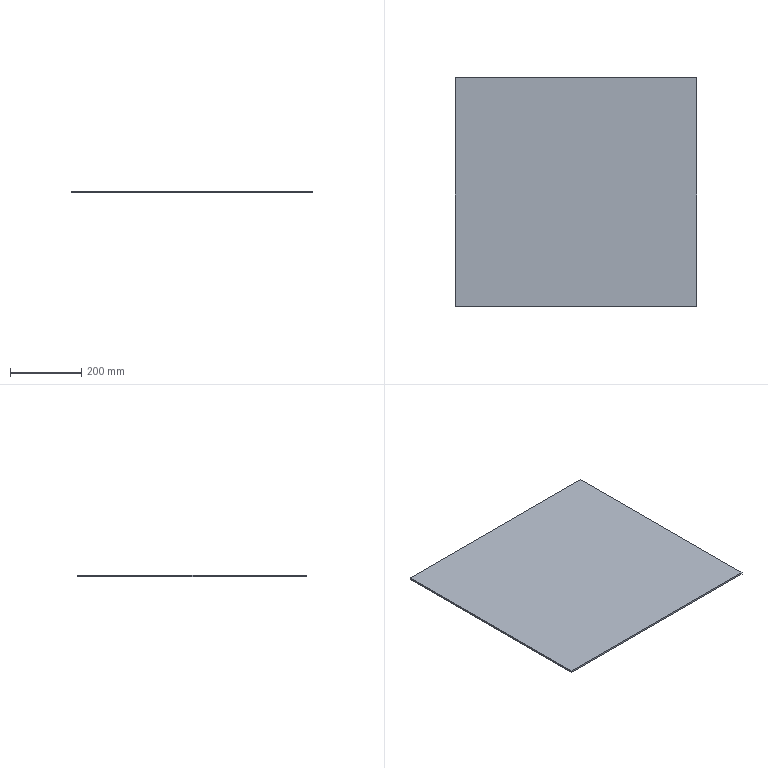Part | SolidWorks | features Extrusion 1 | 1 solid | 6 faces | box 676 x 639 x 5 mm | volume 2159820 mm3 | plane 6
STEP:
#1=CARTESIAN_POINT('',(338.,-319.5,0.));
#2=VERTEX_POINT('',#1);
#3=CARTESIAN_POINT('',(338.,319.5,0.));
#4=VERTEX_POINT('',#3);
#5=CARTESIAN_POINT('',(338.,319.5,0.));
#6=DIRECTION('',(0.,1.,0.));
#7=VECTOR('',#6,1000.);
#8=LINE('',#5,#7);
#9=EDGE_CURVE('',#2,#4,#8,.T.);
#10=ORIENTED_EDGE('',*,*,#9,.T.);
#11=CARTESIAN_POINT('',(338.,319.5,5.));
#12=VERTEX_POINT('',#11);
#13=CARTESIAN_POINT('',(338.,319.5,5.));
#14=DIRECTION('',(0.,0.,-1.));
#15=VECTOR('',#14,1000.);
#16=LINE('',#13,#15);
#17=EDGE_CURVE('',#12,#4,#16,.T.);
#18=ORIENTED_EDGE('',*,*,#17,.F.);
#19=CARTESIAN_POINT('',(338.,-319.5,5.));
#20=VERTEX_POINT('',#19);
#21=CARTESIAN_POINT('',(338.,319.5,5.));
#22=DIRECTION('',(0.,1.,0.));
#23=VECTOR('',#22,1000.);
#24=LINE('',#21,#23);
#25=EDGE_CURVE('',#20,#12,#24,.T.);
#26=ORIENTED_EDGE('',*,*,#25,.F.);
#27=CARTESIAN_POINT('',(338.,-319.5,5.));
#28=DIRECTION('',(0.,0.,-1.));
#29=VECTOR('',#28,1000.);
#30=LINE('',#27,#29);
#31=EDGE_CURVE('',#20,#2,#30,.T.);
#32=ORIENTED_EDGE('',*,*,#31,.T.);
#33=EDGE_LOOP('',(#10,#18,#26,#32));
#34=FACE_OUTER_BOUND('',#33,.T.);
#35=CARTESIAN_POINT('',(338.,319.5,5.));
#36=DIRECTION('',(-1.,0.,0.));
#37=DIRECTION('',(0.,-1.,0.));
#38=AXIS2_PLACEMENT_3D('',#35,#36,#37);
#39=PLANE('',#38);
#40=ADVANCED_FACE('',(#34),#39,.F.);
#41=CARTESIAN_POINT('',(-338.,319.5,0.));
#42=VERTEX_POINT('',#41);
#43=CARTESIAN_POINT('',(-338.,319.5,0.));
#44=DIRECTION('',(-1.,0.,0.));
#45=VECTOR('',#44,1000.);
#46=LINE('',#43,#45);
#47=EDGE_CURVE('',#4,#42,#46,.T.);
#48=ORIENTED_EDGE('',*,*,#47,.T.);
#49=CARTESIAN_POINT('',(-338.,319.5,5.));
#50=VERTEX_POINT('',#49);
#51=CARTESIAN_POINT('',(-338.,319.5,5.));
#52=DIRECTION('',(0.,0.,-1.));
#53=VECTOR('',#52,1000.);
#54=LINE('',#51,#53);
#55=EDGE_CURVE('',#50,#42,#54,.T.);
#56=ORIENTED_EDGE('',*,*,#55,.F.);
#57=CARTESIAN_POINT('',(-338.,319.5,5.));
#58=DIRECTION('',(-1.,0.,0.));
#59=VECTOR('',#58,1000.);
#60=LINE('',#57,#59);
#61=EDGE_CURVE('',#12,#50,#60,.T.);
#62=ORIENTED_EDGE('',*,*,#61,.F.);
#63=ORIENTED_EDGE('',*,*,#17,.T.);
#64=EDGE_LOOP('',(#48,#56,#62,#63));
#65=FACE_OUTER_BOUND('',#64,.T.);
#66=CARTESIAN_POINT('',(-338.,319.5,5.));
#67=DIRECTION('',(0.,-1.,0.));
#68=DIRECTION('',(0.,0.,-1.));
#69=AXIS2_PLACEMENT_3D('',#66,#67,#68);
#70=PLANE('',#69);
#71=ADVANCED_FACE('',(#65),#70,.F.);
#72=CARTESIAN_POINT('',(-338.,-319.5,0.));
#73=VERTEX_POINT('',#72);
#74=CARTESIAN_POINT('',(-338.,319.5,0.));
#75=DIRECTION('',(0.,-1.,0.));
#76=VECTOR('',#75,1000.);
#77=LINE('',#74,#76);
#78=EDGE_CURVE('',#42,#73,#77,.T.);
#79=ORIENTED_EDGE('',*,*,#78,.T.);
#80=CARTESIAN_POINT('',(-338.,-319.5,5.));
#81=VERTEX_POINT('',#80);
#82=CARTESIAN_POINT('',(-338.,-319.5,5.));
#83=DIRECTION('',(0.,0.,-1.));
#84=VECTOR('',#83,1000.);
#85=LINE('',#82,#84);
#86=EDGE_CURVE('',#81,#73,#85,.T.);
#87=ORIENTED_EDGE('',*,*,#86,.F.);
#88=CARTESIAN_POINT('',(-338.,319.5,5.));
#89=DIRECTION('',(0.,-1.,0.));
#90=VECTOR('',#89,1000.);
#91=LINE('',#88,#90);
#92=EDGE_CURVE('',#50,#81,#91,.T.);
#93=ORIENTED_EDGE('',*,*,#92,.F.);
#94=ORIENTED_EDGE('',*,*,#55,.T.);
#95=EDGE_LOOP('',(#79,#87,#93,#94));
#96=FACE_OUTER_BOUND('',#95,.T.);
#97=CARTESIAN_POINT('',(-338.,319.5,5.));
#98=DIRECTION('',(1.,0.,0.));
#99=DIRECTION('',(0.,0.,-1.));
#100=AXIS2_PLACEMENT_3D('',#97,#98,#99);
#101=PLANE('',#100);
#102=ADVANCED_FACE('',(#96),#101,.F.);
#103=CARTESIAN_POINT('',(-338.,-319.5,0.));
#104=DIRECTION('',(1.,0.,0.));
#105=VECTOR('',#104,1000.);
#106=LINE('',#103,#105);
#107=EDGE_CURVE('',#73,#2,#106,.T.);
#108=ORIENTED_EDGE('',*,*,#107,.T.);
#109=ORIENTED_EDGE('',*,*,#31,.F.);
#110=CARTESIAN_POINT('',(-338.,-319.5,5.));
#111=DIRECTION('',(1.,0.,0.));
#112=VECTOR('',#111,1000.);
#113=LINE('',#110,#112);
#114=EDGE_CURVE('',#81,#20,#113,.T.);
#115=ORIENTED_EDGE('',*,*,#114,.F.);
#116=ORIENTED_EDGE('',*,*,#86,.T.);
#117=EDGE_LOOP('',(#108,#109,#115,#116));
#118=FACE_OUTER_BOUND('',#117,.T.);
#119=CARTESIAN_POINT('',(-338.,-319.5,5.));
#120=DIRECTION('',(0.,1.,0.));
#121=DIRECTION('',(0.,0.,1.));
#122=AXIS2_PLACEMENT_3D('',#119,#120,#121);
#123=PLANE('',#122);
#124=ADVANCED_FACE('',(#118),#123,.F.);
#125=ORIENTED_EDGE('',*,*,#25,.T.);
#126=ORIENTED_EDGE('',*,*,#61,.T.);
#127=ORIENTED_EDGE('',*,*,#92,.T.);
#128=ORIENTED_EDGE('',*,*,#114,.T.);
#129=EDGE_LOOP('',(#125,#126,#127,#128));
#130=FACE_OUTER_BOUND('',#129,.T.);
#131=CARTESIAN_POINT('',(0.,0.,5.));
#132=DIRECTION('',(0.,0.,1.));
#133=DIRECTION('',(1.,0.,0.));
#134=AXIS2_PLACEMENT_3D('',#131,#132,#133);
#135=PLANE('',#134);
#136=ADVANCED_FACE('',(#130),#135,.T.);
#137=ORIENTED_EDGE('',*,*,#9,.F.);
#138=ORIENTED_EDGE('',*,*,#107,.F.);
#139=ORIENTED_EDGE('',*,*,#78,.F.);
#140=ORIENTED_EDGE('',*,*,#47,.F.);
#141=EDGE_LOOP('',(#137,#138,#139,#140));
#142=FACE_OUTER_BOUND('',#141,.T.);
#143=CARTESIAN_POINT('',(0.,0.,0.));
#144=DIRECTION('',(0.,0.,1.));
#145=DIRECTION('',(1.,0.,0.));
#146=AXIS2_PLACEMENT_3D('',#143,#144,#145);
#147=PLANE('',#146);
#148=ADVANCED_FACE('',(#142),#147,.F.);
#149=CLOSED_SHELL('',(#40,#71,#102,#124,#136,#148));
#150=MANIFOLD_SOLID_BREP('',#149);
#151=CARTESIAN_POINT('',(0.,0.,0.));
#152=DIRECTION('',(0.,0.,1.));
#153=DIRECTION('',(1.,0.,0.));
#154=AXIS2_PLACEMENT_3D('',#151,#152,#153);
#155=(LENGTH_UNIT()NAMED_UNIT(*)SI_UNIT(.MILLI.,.METRE.));
#156=UNCERTAINTY_MEASURE_WITH_UNIT(LENGTH_MEASURE(0.00001),#155,'','');
#157=(NAMED_UNIT(*)PLANE_ANGLE_UNIT()SI_UNIT($,.RADIAN.));
#158=(NAMED_UNIT(*)SI_UNIT($,.STERADIAN.)SOLID_ANGLE_UNIT());
#159=(GEOMETRIC_REPRESENTATION_CONTEXT(3)GLOBAL_UNCERTAINTY_ASSIGNED_CONTEXT((#156))GLOBAL_UNIT_ASSIGNED_CONTEXT((#155,#157,#158))REPRESENTATION_CONTEXT('',''));
#160=ADVANCED_BREP_SHAPE_REPRESENTATION('',(#150,#154),#159);